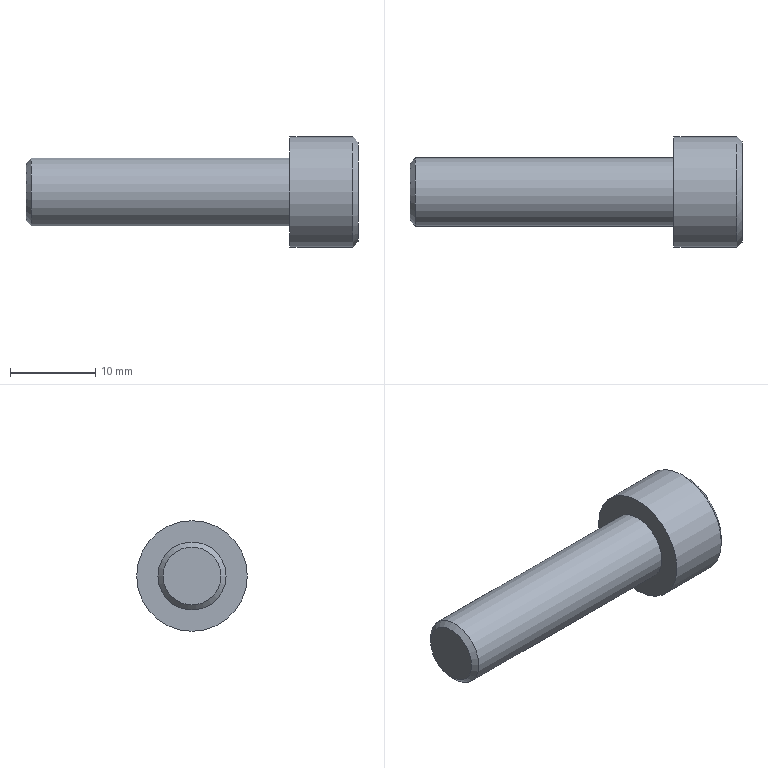Part | STEP file | solid 249 | 1 solid | 14 faces | box 39 x 13 x 13 mm | volume 2484 mm3 | plane 10 | cylinder 2 | cone 2 | commonest cylinder face diameters 8 x1 13 x1